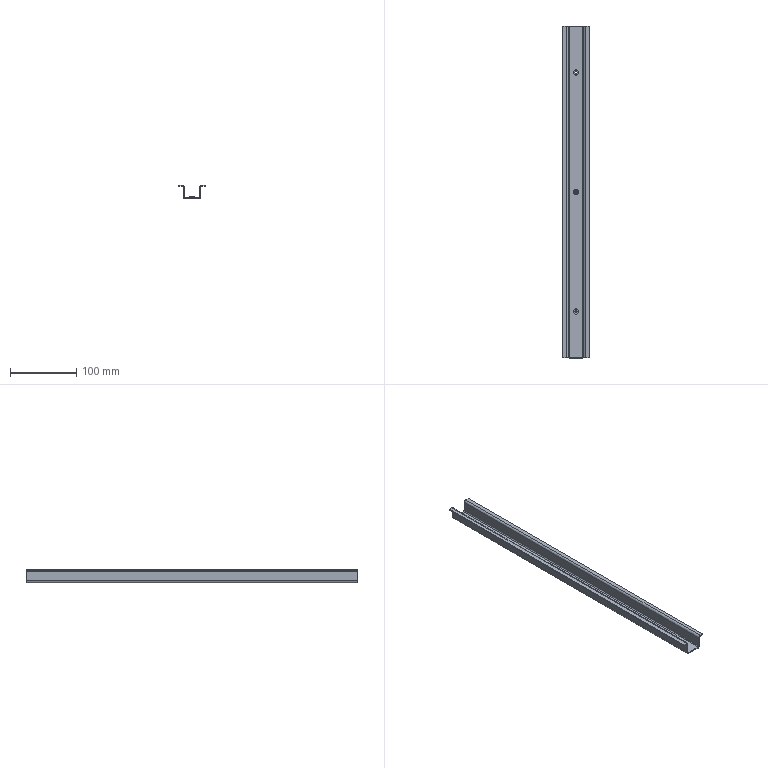Part | SolidWorks | features 3DProfileFeature 1, FlatPattern 1, HoleWzd 1, ICE 1, SMBaseFlange 1, SheetMetal 1 | 1 solid | 53 faces | box 40 x 500 x 21 mm | volume 56565 mm3 | plane 33 | cylinder 20 | commonest cylinder face diameters 3.3 x6 8 x6 3 x4 6 x4
STEP:
#1=CARTESIAN_POINT('',(-1.65,180.,-19.5));
#2=VERTEX_POINT('',#1);
#3=CARTESIAN_POINT('',(1.65,180.,-19.5));
#4=VERTEX_POINT('',#3);
#5=CARTESIAN_POINT('',(0.,180.,-19.5));
#6=DIRECTION('',(0.,0.,1.));
#7=DIRECTION('',(1.,0.,0.));
#8=AXIS2_PLACEMENT_3D('',#5,#6,#7);
#9=CIRCLE('',#8,1.65);
#10=EDGE_CURVE('',#2,#4,#9,.T.);
#11=ORIENTED_EDGE('',*,*,#10,.F.);
#12=CARTESIAN_POINT('',(-1.65,180.,-16.));
#13=VERTEX_POINT('',#12);
#14=CARTESIAN_POINT('',(-1.65,180.,-16.));
#15=DIRECTION('',(0.,0.,1.));
#16=VECTOR('',#15,1000.);
#17=LINE('',#14,#16);
#18=EDGE_CURVE('',#2,#13,#17,.T.);
#19=ORIENTED_EDGE('',*,*,#18,.T.);
#20=CARTESIAN_POINT('',(1.65,180.,-16.));
#21=VERTEX_POINT('',#20);
#22=CARTESIAN_POINT('',(0.,180.,-16.));
#23=DIRECTION('',(0.,0.,1.));
#24=DIRECTION('',(1.,0.,0.));
#25=AXIS2_PLACEMENT_3D('',#22,#23,#24);
#26=CIRCLE('',#25,1.65);
#27=EDGE_CURVE('',#13,#21,#26,.T.);
#28=ORIENTED_EDGE('',*,*,#27,.T.);
#29=CARTESIAN_POINT('',(1.65,180.,-16.));
#30=DIRECTION('',(0.,0.,1.));
#31=VECTOR('',#30,1000.);
#32=LINE('',#29,#31);
#33=EDGE_CURVE('',#4,#21,#32,.T.);
#34=ORIENTED_EDGE('',*,*,#33,.F.);
#35=EDGE_LOOP('',(#11,#19,#28,#34));
#36=FACE_OUTER_BOUND('',#35,.T.);
#37=CARTESIAN_POINT('',(0.,180.,-16.));
#38=DIRECTION('',(0.,0.,1.));
#39=DIRECTION('',(1.,0.,0.));
#40=AXIS2_PLACEMENT_3D('',#37,#38,#39);
#41=CYLINDRICAL_SURFACE('',#40,1.65);
#42=ADVANCED_FACE('',(#36),#41,.F.);
#43=CARTESIAN_POINT('',(-1.65,0.,-19.5));
#44=VERTEX_POINT('',#43);
#45=CARTESIAN_POINT('',(1.65,0.,-19.5));
#46=VERTEX_POINT('',#45);
#47=CARTESIAN_POINT('',(0.,0.,-19.5));
#48=DIRECTION('',(0.,0.,1.));
#49=DIRECTION('',(1.,0.,0.));
#50=AXIS2_PLACEMENT_3D('',#47,#48,#49);
#51=CIRCLE('',#50,1.65);
#52=EDGE_CURVE('',#44,#46,#51,.T.);
#53=ORIENTED_EDGE('',*,*,#52,.F.);
#54=CARTESIAN_POINT('',(-1.65,0.,-16.));
#55=VERTEX_POINT('',#54);
#56=CARTESIAN_POINT('',(-1.65,0.,-16.));
#57=DIRECTION('',(0.,0.,1.));
#58=VECTOR('',#57,1000.);
#59=LINE('',#56,#58);
#60=EDGE_CURVE('',#44,#55,#59,.T.);
#61=ORIENTED_EDGE('',*,*,#60,.T.);
#62=CARTESIAN_POINT('',(1.65,0.,-16.));
#63=VERTEX_POINT('',#62);
#64=CARTESIAN_POINT('',(0.,0.,-16.));
#65=DIRECTION('',(0.,0.,1.));
#66=DIRECTION('',(1.,0.,0.));
#67=AXIS2_PLACEMENT_3D('',#64,#65,#66);
#68=CIRCLE('',#67,1.65);
#69=EDGE_CURVE('',#55,#63,#68,.T.);
#70=ORIENTED_EDGE('',*,*,#69,.T.);
#71=CARTESIAN_POINT('',(1.65,0.,-16.));
#72=DIRECTION('',(0.,0.,1.));
#73=VECTOR('',#72,1000.);
#74=LINE('',#71,#73);
#75=EDGE_CURVE('',#46,#63,#74,.T.);
#76=ORIENTED_EDGE('',*,*,#75,.F.);
#77=EDGE_LOOP('',(#53,#61,#70,#76));
#78=FACE_OUTER_BOUND('',#77,.T.);
#79=CARTESIAN_POINT('',(0.,0.,-16.));
#80=DIRECTION('',(0.,0.,1.));
#81=DIRECTION('',(1.,0.,0.));
#82=AXIS2_PLACEMENT_3D('',#79,#80,#81);
#83=CYLINDRICAL_SURFACE('',#82,1.65);
#84=ADVANCED_FACE('',(#78),#83,.F.);
#85=CARTESIAN_POINT('',(-1.65,-180.,-19.5));
#86=VERTEX_POINT('',#85);
#87=CARTESIAN_POINT('',(1.65,-180.,-19.5));
#88=VERTEX_POINT('',#87);
#89=CARTESIAN_POINT('',(0.,-180.,-19.5));
#90=DIRECTION('',(0.,0.,1.));
#91=DIRECTION('',(1.,0.,0.));
#92=AXIS2_PLACEMENT_3D('',#89,#90,#91);
#93=CIRCLE('',#92,1.65);
#94=EDGE_CURVE('',#86,#88,#93,.T.);
#95=ORIENTED_EDGE('',*,*,#94,.F.);
#96=CARTESIAN_POINT('',(-1.65,-180.,-16.));
#97=VERTEX_POINT('',#96);
#98=CARTESIAN_POINT('',(-1.65,-180.,-16.));
#99=DIRECTION('',(0.,0.,1.));
#100=VECTOR('',#99,1000.);
#101=LINE('',#98,#100);
#102=EDGE_CURVE('',#86,#97,#101,.T.);
#103=ORIENTED_EDGE('',*,*,#102,.T.);
#104=CARTESIAN_POINT('',(1.65,-180.,-16.));
#105=VERTEX_POINT('',#104);
#106=CARTESIAN_POINT('',(0.,-180.,-16.));
#107=DIRECTION('',(0.,0.,1.));
#108=DIRECTION('',(1.,0.,0.));
#109=AXIS2_PLACEMENT_3D('',#106,#107,#108);
#110=CIRCLE('',#109,1.65);
#111=EDGE_CURVE('',#97,#105,#110,.T.);
#112=ORIENTED_EDGE('',*,*,#111,.T.);
#113=CARTESIAN_POINT('',(1.65,-180.,-16.));
#114=DIRECTION('',(0.,0.,1.));
#115=VECTOR('',#114,1000.);
#116=LINE('',#113,#115);
#117=EDGE_CURVE('',#88,#105,#116,.T.);
#118=ORIENTED_EDGE('',*,*,#117,.F.);
#119=EDGE_LOOP('',(#95,#103,#112,#118));
#120=FACE_OUTER_BOUND('',#119,.T.);
#121=CARTESIAN_POINT('',(0.,-180.,-16.));
#122=DIRECTION('',(0.,0.,1.));
#123=DIRECTION('',(1.,0.,0.));
#124=AXIS2_PLACEMENT_3D('',#121,#122,#123);
#125=CYLINDRICAL_SURFACE('',#124,1.65);
#126=ADVANCED_FACE('',(#120),#125,.F.);
#127=CARTESIAN_POINT('',(-4.,-180.,-16.));
#128=VERTEX_POINT('',#127);
#129=CARTESIAN_POINT('',(4.,-180.,-16.));
#130=VERTEX_POINT('',#129);
#131=CARTESIAN_POINT('',(0.,-180.,-16.));
#132=DIRECTION('',(0.,0.,-1.));
#133=DIRECTION('',(1.,0.,0.));
#134=AXIS2_PLACEMENT_3D('',#131,#132,#133);
#135=CIRCLE('',#134,4.);
#136=EDGE_CURVE('',#128,#130,#135,.T.);
#137=ORIENTED_EDGE('',*,*,#136,.T.);
#138=CARTESIAN_POINT('',(4.,-180.,-18.));
#139=VERTEX_POINT('',#138);
#140=CARTESIAN_POINT('',(4.,-180.,-16.));
#141=DIRECTION('',(0.,0.,-1.));
#142=VECTOR('',#141,1000.);
#143=LINE('',#140,#142);
#144=EDGE_CURVE('',#130,#139,#143,.T.);
#145=ORIENTED_EDGE('',*,*,#144,.T.);
#146=CARTESIAN_POINT('',(-4.,-180.,-18.));
#147=VERTEX_POINT('',#146);
#148=CARTESIAN_POINT('',(0.,-180.,-18.));
#149=DIRECTION('',(0.,0.,-1.));
#150=DIRECTION('',(1.,0.,0.));
#151=AXIS2_PLACEMENT_3D('',#148,#149,#150);
#152=CIRCLE('',#151,4.);
#153=EDGE_CURVE('',#147,#139,#152,.T.);
#154=ORIENTED_EDGE('',*,*,#153,.F.);
#155=CARTESIAN_POINT('',(-4.,-180.,-16.));
#156=DIRECTION('',(0.,0.,-1.));
#157=VECTOR('',#156,1000.);
#158=LINE('',#155,#157);
#159=EDGE_CURVE('',#128,#147,#158,.T.);
#160=ORIENTED_EDGE('',*,*,#159,.F.);
#161=EDGE_LOOP('',(#137,#145,#154,#160));
#162=FACE_OUTER_BOUND('',#161,.T.);
#163=CARTESIAN_POINT('',(0.,-180.,-16.));
#164=DIRECTION('',(0.,0.,-1.));
#165=DIRECTION('',(-1.,0.,0.));
#166=AXIS2_PLACEMENT_3D('',#163,#164,#165);
#167=CYLINDRICAL_SURFACE('',#166,4.);
#168=ADVANCED_FACE('',(#162),#167,.T.);
#169=CARTESIAN_POINT('',(4.,0.,-16.));
#170=VERTEX_POINT('',#169);
#171=CARTESIAN_POINT('',(-4.,0.,-16.));
#172=VERTEX_POINT('',#171);
#173=CARTESIAN_POINT('',(0.,0.,-16.));
#174=DIRECTION('',(0.,0.,1.));
#175=DIRECTION('',(1.,0.,0.));
#176=AXIS2_PLACEMENT_3D('',#173,#174,#175);
#177=CIRCLE('',#176,4.);
#178=EDGE_CURVE('',#170,#172,#177,.T.);
#179=ORIENTED_EDGE('',*,*,#178,.F.);
#180=CARTESIAN_POINT('',(4.,0.,-18.));
#181=VERTEX_POINT('',#180);
#182=CARTESIAN_POINT('',(4.,0.,-16.));
#183=DIRECTION('',(0.,0.,-1.));
#184=VECTOR('',#183,1000.);
#185=LINE('',#182,#184);
#186=EDGE_CURVE('',#170,#181,#185,.T.);
#187=ORIENTED_EDGE('',*,*,#186,.T.);
#188=CARTESIAN_POINT('',(-4.,0.,-18.));
#189=VERTEX_POINT('',#188);
#190=CARTESIAN_POINT('',(0.,0.,-18.));
#191=DIRECTION('',(0.,0.,1.));
#192=DIRECTION('',(-1.,0.,0.));
#193=AXIS2_PLACEMENT_3D('',#190,#191,#192);
#194=CIRCLE('',#193,4.);
#195=EDGE_CURVE('',#181,#189,#194,.T.);
#196=ORIENTED_EDGE('',*,*,#195,.T.);
#197=CARTESIAN_POINT('',(-4.,0.,-16.));
#198=DIRECTION('',(0.,0.,-1.));
#199=VECTOR('',#198,1000.);
#200=LINE('',#197,#199);
#201=EDGE_CURVE('',#172,#189,#200,.T.);
#202=ORIENTED_EDGE('',*,*,#201,.F.);
#203=EDGE_LOOP('',(#179,#187,#196,#202));
#204=FACE_OUTER_BOUND('',#203,.T.);
#205=CARTESIAN_POINT('',(0.,0.,-16.));
#206=DIRECTION('',(0.,0.,-1.));
#207=DIRECTION('',(-1.,0.,0.));
#208=AXIS2_PLACEMENT_3D('',#205,#206,#207);
#209=CYLINDRICAL_SURFACE('',#208,4.);
#210=ADVANCED_FACE('',(#204),#209,.T.);
#211=CARTESIAN_POINT('',(4.,180.,-16.));
#212=VERTEX_POINT('',#211);
#213=CARTESIAN_POINT('',(-4.,180.,-16.));
#214=VERTEX_POINT('',#213);
#215=CARTESIAN_POINT('',(0.,180.,-16.));
#216=DIRECTION('',(0.,0.,1.));
#217=DIRECTION('',(1.,0.,0.));
#218=AXIS2_PLACEMENT_3D('',#215,#216,#217);
#219=CIRCLE('',#218,4.);
#220=EDGE_CURVE('',#212,#214,#219,.T.);
#221=ORIENTED_EDGE('',*,*,#220,.F.);
#222=CARTESIAN_POINT('',(4.,180.,-18.));
#223=VERTEX_POINT('',#222);
#224=CARTESIAN_POINT('',(4.,180.,-16.));
#225=DIRECTION('',(0.,0.,-1.));
#226=VECTOR('',#225,1000.);
#227=LINE('',#224,#226);
#228=EDGE_CURVE('',#212,#223,#227,.T.);
#229=ORIENTED_EDGE('',*,*,#228,.T.);
#230=CARTESIAN_POINT('',(-4.,180.,-18.));
#231=VERTEX_POINT('',#230);
#232=CARTESIAN_POINT('',(0.,180.,-18.));
#233=DIRECTION('',(0.,0.,1.));
#234=DIRECTION('',(-1.,0.,0.));
#235=AXIS2_PLACEMENT_3D('',#232,#233,#234);
#236=CIRCLE('',#235,4.);
#237=EDGE_CURVE('',#223,#231,#236,.T.);
#238=ORIENTED_EDGE('',*,*,#237,.T.);
#239=CARTESIAN_POINT('',(-4.,180.,-16.));
#240=DIRECTION('',(0.,0.,-1.));
#241=VECTOR('',#240,1000.);
#242=LINE('',#239,#241);
#243=EDGE_CURVE('',#214,#231,#242,.T.);
#244=ORIENTED_EDGE('',*,*,#243,.F.);
#245=EDGE_LOOP('',(#221,#229,#238,#244));
#246=FACE_OUTER_BOUND('',#245,.T.);
#247=CARTESIAN_POINT('',(0.,180.,-16.));
#248=DIRECTION('',(0.,0.,-1.));
#249=DIRECTION('',(-1.,0.,0.));
#250=AXIS2_PLACEMENT_3D('',#247,#248,#249);
#251=CYLINDRICAL_SURFACE('',#250,4.);
#252=ADVANCED_FACE('',(#246),#251,.T.);
#253=CARTESIAN_POINT('',(-13.,250.,-1.5));
#254=VERTEX_POINT('',#253);
#255=CARTESIAN_POINT('',(-11.5,250.,-1.5));
#256=VERTEX_POINT('',#255);
#257=CARTESIAN_POINT('',(-13.,250.,-1.5));
#258=DIRECTION('',(1.,0.,0.));
#259=VECTOR('',#258,1000.);
#260=LINE('',#257,#259);
#261=EDGE_CURVE('',#254,#256,#260,.T.);
#262=ORIENTED_EDGE('',*,*,#261,.F.);
#263=CARTESIAN_POINT('',(-14.5,250.,0.));
#264=VERTEX_POINT('',#263);
#265=CARTESIAN_POINT('',(-14.5,250.,-1.5));
#266=DIRECTION('',(0.,1.,0.));
#267=DIRECTION('',(0.,0.,-1.));
#268=AXIS2_PLACEMENT_3D('',#265,#266,#267);
#269=CIRCLE('',#268,1.5);
#270=EDGE_CURVE('',#264,#254,#269,.T.);
#271=ORIENTED_EDGE('',*,*,#270,.F.);
#272=CARTESIAN_POINT('',(-14.5,250.,1.5));
#273=VERTEX_POINT('',#272);
#274=CARTESIAN_POINT('',(-14.5,250.,1.5));
#275=DIRECTION('',(0.,0.,-1.));
#276=VECTOR('',#275,1000.);
#277=LINE('',#274,#276);
#278=EDGE_CURVE('',#273,#264,#277,.T.);
#279=ORIENTED_EDGE('',*,*,#278,.F.);
#280=CARTESIAN_POINT('',(-14.5,250.,-1.5));
#281=DIRECTION('',(0.,1.,0.));
#282=DIRECTION('',(1.,0.,0.));
#283=AXIS2_PLACEMENT_3D('',#280,#281,#282);
#284=CIRCLE('',#283,3.);
#285=EDGE_CURVE('',#273,#256,#284,.T.);
#286=ORIENTED_EDGE('',*,*,#285,.T.);
#287=EDGE_LOOP('',(#262,#271,#279,#286));
#288=FACE_OUTER_BOUND('',#287,.T.);
#289=CARTESIAN_POINT('',(-13.,250.,-1.5));
#290=DIRECTION('',(0.,1.,0.));
#291=DIRECTION('',(0.,0.,1.));
#292=AXIS2_PLACEMENT_3D('',#289,#290,#291);
#293=PLANE('',#292);
#294=ADVANCED_FACE('',(#288),#293,.T.);
#295=CARTESIAN_POINT('',(-13.,250.,-16.5));
#296=VERTEX_POINT('',#295);
#297=CARTESIAN_POINT('',(-13.,250.,0.));
#298=DIRECTION('',(0.,0.,-1.));
#299=VECTOR('',#298,1000.);
#300=LINE('',#297,#299);
#301=EDGE_CURVE('',#254,#296,#300,.T.);
#302=ORIENTED_EDGE('',*,*,#301,.F.);
#303=ORIENTED_EDGE('',*,*,#261,.T.);
#304=CARTESIAN_POINT('',(-11.5,250.,-16.5));
#305=VERTEX_POINT('',#304);
#306=CARTESIAN_POINT('',(-11.5,250.,0.));
#307=DIRECTION('',(0.,0.,-1.));
#308=VECTOR('',#307,1000.);
#309=LINE('',#306,#308);
#310=EDGE_CURVE('',#256,#305,#309,.T.);
#311=ORIENTED_EDGE('',*,*,#310,.T.);
#312=CARTESIAN_POINT('',(-11.5,250.,-16.5));
#313=DIRECTION('',(-1.,0.,0.));
#314=VECTOR('',#313,1000.);
#315=LINE('',#312,#314);
#316=EDGE_CURVE('',#305,#296,#315,.T.);
#317=ORIENTED_EDGE('',*,*,#316,.T.);
#318=EDGE_LOOP('',(#302,#303,#311,#317));
#319=FACE_OUTER_BOUND('',#318,.T.);
#320=CARTESIAN_POINT('',(-14.5,250.,1.5));
#321=DIRECTION('',(0.,1.,0.));
#322=DIRECTION('',(0.,0.,1.));
#323=AXIS2_PLACEMENT_3D('',#320,#321,#322);
#324=PLANE('',#323);
#325=ADVANCED_FACE('',(#319),#324,.T.);
#326=CARTESIAN_POINT('',(-14.5,-250.,0.));
#327=VERTEX_POINT('',#326);
#328=CARTESIAN_POINT('',(-14.5,-250.,1.5));
#329=VERTEX_POINT('',#328);
#330=CARTESIAN_POINT('',(-14.5,-250.,0.));
#331=DIRECTION('',(0.,0.,1.));
#332=VECTOR('',#331,1000.);
#333=LINE('',#330,#332);
#334=EDGE_CURVE('',#327,#329,#333,.T.);
#335=ORIENTED_EDGE('',*,*,#334,.F.);
#336=CARTESIAN_POINT('',(-13.,-250.,-1.5));
#337=VERTEX_POINT('',#336);
#338=CARTESIAN_POINT('',(-14.5,-250.,-1.5));
#339=DIRECTION('',(0.,1.,0.));
#340=DIRECTION('',(0.,0.,-1.));
#341=AXIS2_PLACEMENT_3D('',#338,#339,#340);
#342=CIRCLE('',#341,1.5);
#343=EDGE_CURVE('',#327,#337,#342,.T.);
#344=ORIENTED_EDGE('',*,*,#343,.T.);
#345=CARTESIAN_POINT('',(-11.5,-250.,-1.5));
#346=VERTEX_POINT('',#345);
#347=CARTESIAN_POINT('',(-11.5,-250.,-1.5));
#348=DIRECTION('',(-1.,0.,0.));
#349=VECTOR('',#348,1000.);
#350=LINE('',#347,#349);
#351=EDGE_CURVE('',#346,#337,#350,.T.);
#352=ORIENTED_EDGE('',*,*,#351,.F.);
#353=CARTESIAN_POINT('',(-14.5,-250.,-1.5));
#354=DIRECTION('',(0.,1.,0.));
#355=DIRECTION('',(1.,0.,0.));
#356=AXIS2_PLACEMENT_3D('',#353,#354,#355);
#357=CIRCLE('',#356,3.);
#358=EDGE_CURVE('',#329,#346,#357,.T.);
#359=ORIENTED_EDGE('',*,*,#358,.F.);
#360=EDGE_LOOP('',(#335,#344,#352,#359));
#361=FACE_OUTER_BOUND('',#360,.T.);
#362=CARTESIAN_POINT('',(-14.5,-250.,0.));
#363=DIRECTION('',(0.,-1.,0.));
#364=DIRECTION('',(0.,0.,-1.));
#365=AXIS2_PLACEMENT_3D('',#362,#363,#364);
#366=PLANE('',#365);
#367=ADVANCED_FACE('',(#361),#366,.T.);
#368=CARTESIAN_POINT('',(-20.,-250.,0.));
#369=VERTEX_POINT('',#368);
#370=CARTESIAN_POINT('',(-20.,-250.,0.));
#371=DIRECTION('',(1.,0.,0.));
#372=VECTOR('',#371,1000.);
#373=LINE('',#370,#372);
#374=EDGE_CURVE('',#369,#327,#373,.T.);
#375=ORIENTED_EDGE('',*,*,#374,.T.);
#376=ORIENTED_EDGE('',*,*,#334,.T.);
#377=CARTESIAN_POINT('',(-20.,-250.,1.5));
#378=VERTEX_POINT('',#377);
#379=CARTESIAN_POINT('',(-20.,-250.,1.5));
#380=DIRECTION('',(1.,0.,0.));
#381=VECTOR('',#380,1000.);
#382=LINE('',#379,#381);
#383=EDGE_CURVE('',#378,#329,#382,.T.);
#384=ORIENTED_EDGE('',*,*,#383,.F.);
#385=CARTESIAN_POINT('',(-20.,-250.,1.5));
#386=DIRECTION('',(0.,0.,-1.));
#387=VECTOR('',#386,1000.);
#388=LINE('',#385,#387);
#389=EDGE_CURVE('',#378,#369,#388,.T.);
#390=ORIENTED_EDGE('',*,*,#389,.T.);
#391=EDGE_LOOP('',(#375,#376,#384,#390));
#392=FACE_OUTER_BOUND('',#391,.T.);
#393=CARTESIAN_POINT('',(-11.5,-250.,-1.5));
#394=DIRECTION('',(0.,-1.,0.));
#395=DIRECTION('',(0.,0.,-1.));
#396=AXIS2_PLACEMENT_3D('',#393,#394,#395);
#397=PLANE('',#396);
#398=ADVANCED_FACE('',(#392),#397,.T.);
#399=CARTESIAN_POINT('',(-10.,250.,-19.5));
#400=VERTEX_POINT('',#399);
#401=CARTESIAN_POINT('',(-10.,250.,-18.));
#402=VERTEX_POINT('',#401);
#403=CARTESIAN_POINT('',(-10.,250.,-19.5));
#404=DIRECTION('',(0.,0.,1.));
#405=VECTOR('',#404,1000.);
#406=LINE('',#403,#405);
#407=EDGE_CURVE('',#400,#402,#406,.T.);
#408=ORIENTED_EDGE('',*,*,#407,.F.);
#409=CARTESIAN_POINT('',(-10.,250.,-16.5));
#410=DIRECTION('',(0.,-1.,0.));
#411=DIRECTION('',(0.,0.,1.));
#412=AXIS2_PLACEMENT_3D('',#409,#410,#411);
#413=CIRCLE('',#412,3.);
#414=EDGE_CURVE('',#296,#400,#413,.T.);
#415=ORIENTED_EDGE('',*,*,#414,.F.);
#416=ORIENTED_EDGE('',*,*,#316,.F.);
#417=CARTESIAN_POINT('',(-10.,250.,-16.5));
#418=DIRECTION('',(0.,-1.,0.));
#419=DIRECTION('',(1.,0.,0.));
#420=AXIS2_PLACEMENT_3D('',#417,#418,#419);
#421=CIRCLE('',#420,1.5);
#422=EDGE_CURVE('',#305,#402,#421,.T.);
#423=ORIENTED_EDGE('',*,*,#422,.T.);
#424=EDGE_LOOP('',(#408,#415,#416,#423));
#425=FACE_OUTER_BOUND('',#424,.T.);
#426=CARTESIAN_POINT('',(-10.,250.,-19.5));
#427=DIRECTION('',(0.,1.,0.));
#428=DIRECTION('',(0.,0.,1.));
#429=AXIS2_PLACEMENT_3D('',#426,#427,#428);
#430=PLANE('',#429);
#431=ADVANCED_FACE('',(#425),#430,.T.);
#432=CARTESIAN_POINT('',(10.,250.,-19.5));
#433=VERTEX_POINT('',#432);
#434=CARTESIAN_POINT('',(-13.,250.,-19.5));
#435=DIRECTION('',(1.,0.,0.));
#436=VECTOR('',#435,1000.);
#437=LINE('',#434,#436);
#438=EDGE_CURVE('',#400,#433,#437,.T.);
#439=ORIENTED_EDGE('',*,*,#438,.F.);
#440=ORIENTED_EDGE('',*,*,#407,.T.);
#441=CARTESIAN_POINT('',(10.,250.,-18.));
#442=VERTEX_POINT('',#441);
#443=CARTESIAN_POINT('',(-13.,250.,-18.));
#444=DIRECTION('',(1.,0.,0.));
#445=VECTOR('',#444,1000.);
#446=LINE('',#443,#445);
#447=EDGE_CURVE('',#402,#442,#446,.T.);
#448=ORIENTED_EDGE('',*,*,#447,.T.);
#449=CARTESIAN_POINT('',(10.,250.,-18.));
#450=DIRECTION('',(0.,0.,-1.));
#451=VECTOR('',#450,1000.);
#452=LINE('',#449,#451);
#453=EDGE_CURVE('',#442,#433,#452,.T.);
#454=ORIENTED_EDGE('',*,*,#453,.T.);
#455=EDGE_LOOP('',(#439,#440,#448,#454));
#456=FACE_OUTER_BOUND('',#455,.T.);
#457=CARTESIAN_POINT('',(-11.5,250.,-16.5));
#458=DIRECTION('',(0.,1.,0.));
#459=DIRECTION('',(0.,0.,1.));
#460=AXIS2_PLACEMENT_3D('',#457,#458,#459);
#461=PLANE('',#460);
#462=ADVANCED_FACE('',(#456),#461,.T.);
#463=CARTESIAN_POINT('',(-13.,-250.,-16.5));
#464=VERTEX_POINT('',#463);
#465=CARTESIAN_POINT('',(-11.5,-250.,-16.5));
#466=VERTEX_POINT('',#465);
#467=CARTESIAN_POINT('',(-13.,-250.,-16.5));
#468=DIRECTION('',(1.,0.,0.));
#469=VECTOR('',#468,1000.);
#470=LINE('',#467,#469);
#471=EDGE_CURVE('',#464,#466,#470,.T.);
#472=ORIENTED_EDGE('',*,*,#471,.F.);
#473=CARTESIAN_POINT('',(-10.,-250.,-19.5));
#474=VERTEX_POINT('',#473);
#475=CARTESIAN_POINT('',(-10.,-250.,-16.5));
#476=DIRECTION('',(0.,-1.,0.));
#477=DIRECTION('',(0.,0.,1.));
#478=AXIS2_PLACEMENT_3D('',#475,#476,#477);
#479=CIRCLE('',#478,3.);
#480=EDGE_CURVE('',#464,#474,#479,.T.);
#481=ORIENTED_EDGE('',*,*,#480,.T.);
#482=CARTESIAN_POINT('',(-10.,-250.,-18.));
#483=VERTEX_POINT('',#482);
#484=CARTESIAN_POINT('',(-10.,-250.,-18.));
#485=DIRECTION('',(0.,0.,-1.));
#486=VECTOR('',#485,1000.);
#487=LINE('',#484,#486);
#488=EDGE_CURVE('',#483,#474,#487,.T.);
#489=ORIENTED_EDGE('',*,*,#488,.F.);
#490=CARTESIAN_POINT('',(-10.,-250.,-16.5));
#491=DIRECTION('',(0.,-1.,0.));
#492=DIRECTION('',(1.,0.,0.));
#493=AXIS2_PLACEMENT_3D('',#490,#491,#492);
#494=CIRCLE('',#493,1.5);
#495=EDGE_CURVE('',#466,#483,#494,.T.);
#496=ORIENTED_EDGE('',*,*,#495,.F.);
#497=EDGE_LOOP('',(#472,#481,#489,#496));
#498=FACE_OUTER_BOUND('',#497,.T.);
#499=CARTESIAN_POINT('',(-13.,-250.,-16.5));
#500=DIRECTION('',(0.,-1.,0.));
#501=DIRECTION('',(0.,0.,-1.));
#502=AXIS2_PLACEMENT_3D('',#499,#500,#501);
#503=PLANE('',#502);
#504=ADVANCED_FACE('',(#498),#503,.T.);
#505=CARTESIAN_POINT('',(-13.,-250.,0.));
#506=DIRECTION('',(0.,0.,-1.));
#507=VECTOR('',#506,1000.);
#508=LINE('',#505,#507);
#509=EDGE_CURVE('',#337,#464,#508,.T.);
#510=ORIENTED_EDGE('',*,*,#509,.T.);
#511=ORIENTED_EDGE('',*,*,#471,.T.);
#512=CARTESIAN_POINT('',(-11.5,-250.,0.));
#513=DIRECTION('',(0.,0.,-1.));
#514=VECTOR('',#513,1000.);
#515=LINE('',#512,#514);
#516=EDGE_CURVE('',#346,#466,#515,.T.);
#517=ORIENTED_EDGE('',*,*,#516,.F.);
#518=ORIENTED_EDGE('',*,*,#351,.T.);
#519=EDGE_LOOP('',(#510,#511,#517,#518));
#520=FACE_OUTER_BOUND('',#519,.T.);
#521=CARTESIAN_POINT('',(-10.,-250.,-18.));
#522=DIRECTION('',(0.,-1.,0.));
#523=DIRECTION('',(0.,0.,-1.));
#524=AXIS2_PLACEMENT_3D('',#521,#522,#523);
#525=PLANE('',#524);
#526=ADVANCED_FACE('',(#520),#525,.T.);
#527=CARTESIAN_POINT('',(13.,250.,-16.5));
#528=VERTEX_POINT('',#527);
#529=CARTESIAN_POINT('',(11.5,250.,-16.5));
#530=VERTEX_POINT('',#529);
#531=CARTESIAN_POINT('',(13.,250.,-16.5));
#532=DIRECTION('',(-1.,0.,0.));
#533=VECTOR('',#532,1000.);
#534=LINE('',#531,#533);
#535=EDGE_CURVE('',#528,#530,#534,.T.);
#536=ORIENTED_EDGE('',*,*,#535,.F.);
#537=CARTESIAN_POINT('',(10.,250.,-16.5));
#538=DIRECTION('',(0.,-1.,0.));
#539=DIRECTION('',(0.,0.,1.));
#540=AXIS2_PLACEMENT_3D('',#537,#538,#539);
#541=CIRCLE('',#540,3.);
#542=EDGE_CURVE('',#433,#528,#541,.T.);
#543=ORIENTED_EDGE('',*,*,#542,.F.);
#544=ORIENTED_EDGE('',*,*,#453,.F.);
#545=CARTESIAN_POINT('',(10.,250.,-16.5));
#546=DIRECTION('',(0.,-1.,0.));
#547=DIRECTION('',(1.,0.,0.));
#548=AXIS2_PLACEMENT_3D('',#545,#546,#547);
#549=CIRCLE('',#548,1.5);
#550=EDGE_CURVE('',#442,#530,#549,.T.);
#551=ORIENTED_EDGE('',*,*,#550,.T.);
#552=EDGE_LOOP('',(#536,#543,#544,#551));
#553=FACE_OUTER_BOUND('',#552,.T.);
#554=CARTESIAN_POINT('',(13.,250.,-16.5));
#555=DIRECTION('',(0.,1.,0.));
#556=DIRECTION('',(0.,0.,1.));
#557=AXIS2_PLACEMENT_3D('',#554,#555,#556);
#558=PLANE('',#557);
#559=ADVANCED_FACE('',(#553),#558,.T.);
#560=CARTESIAN_POINT('',(13.,250.,-1.5));
#561=VERTEX_POINT('',#560);
#562=CARTESIAN_POINT('',(13.,250.,-19.5));
#563=DIRECTION('',(0.,0.,1.));
#564=VECTOR('',#563,1000.);
#565=LINE('',#562,#564);
#566=EDGE_CURVE('',#528,#561,#565,.T.);
#567=ORIENTED_EDGE('',*,*,#566,.F.);
#568=ORIENTED_EDGE('',*,*,#535,.T.);
#569=CARTESIAN_POINT('',(11.5,250.,-1.5));
#570=VERTEX_POINT('',#569);
#571=CARTESIAN_POINT('',(11.5,250.,-19.5));
#572=DIRECTION('',(0.,0.,1.));
#573=VECTOR('',#572,1000.);
#574=LINE('',#571,#573);
#575=EDGE_CURVE('',#530,#570,#574,.T.);
#576=ORIENTED_EDGE('',*,*,#575,.T.);
#577=CARTESIAN_POINT('',(11.5,250.,-1.5));
#578=DIRECTION('',(1.,0.,0.));
#579=VECTOR('',#578,1000.);
#580=LINE('',#577,#579);
#581=EDGE_CURVE('',#570,#561,#580,.T.);
#582=ORIENTED_EDGE('',*,*,#581,.T.);
#583=EDGE_LOOP('',(#567,#568,#576,#582));
#584=FACE_OUTER_BOUND('',#583,.T.);
#585=CARTESIAN_POINT('',(10.,250.,-18.));
#586=DIRECTION('',(0.,1.,0.));
#587=DIRECTION('',(0.,0.,1.));
#588=AXIS2_PLACEMENT_3D('',#585,#586,#587);
#589=PLANE('',#588);
#590=ADVANCED_FACE('',(#584),#589,.T.);
#591=CARTESIAN_POINT('',(10.,-250.,-19.5));
#592=VERTEX_POINT('',#591);
#593=CARTESIAN_POINT('',(10.,-250.,-18.));
#594=VERTEX_POINT('',#593);
#595=CARTESIAN_POINT('',(10.,-250.,-19.5));
#596=DIRECTION('',(0.,0.,1.));
#597=VECTOR('',#596,1000.);
#598=LINE('',#595,#597);
#599=EDGE_CURVE('',#592,#594,#598,.T.);
#600=ORIENTED_EDGE('',*,*,#599,.F.);
#601=CARTESIAN_POINT('',(13.,-250.,-16.5));
#602=VERTEX_POINT('',#601);
#603=CARTESIAN_POINT('',(10.,-250.,-16.5));
#604=DIRECTION('',(0.,-1.,0.));
#605=DIRECTION('',(0.,0.,1.));
#606=AXIS2_PLACEMENT_3D('',#603,#604,#605);
#607=CIRCLE('',#606,3.);
#608=EDGE_CURVE('',#592,#602,#607,.T.);
#609=ORIENTED_EDGE('',*,*,#608,.T.);
#610=CARTESIAN_POINT('',(11.5,-250.,-16.5));
#611=VERTEX_POINT('',#610);
#612=CARTESIAN_POINT('',(11.5,-250.,-16.5));
#613=DIRECTION('',(1.,0.,0.));
#614=VECTOR('',#613,1000.);
#615=LINE('',#612,#614);
#616=EDGE_CURVE('',#611,#602,#615,.T.);
#617=ORIENTED_EDGE('',*,*,#616,.F.);
#618=CARTESIAN_POINT('',(10.,-250.,-16.5));
#619=DIRECTION('',(0.,-1.,0.));
#620=DIRECTION('',(1.,0.,0.));
#621=AXIS2_PLACEMENT_3D('',#618,#619,#620);
#622=CIRCLE('',#621,1.5);
#623=EDGE_CURVE('',#594,#611,#622,.T.);
#624=ORIENTED_EDGE('',*,*,#623,.F.);
#625=EDGE_LOOP('',(#600,#609,#617,#624));
#626=FACE_OUTER_BOUND('',#625,.T.);
#627=CARTESIAN_POINT('',(10.,-250.,-19.5));
#628=DIRECTION('',(0.,-1.,0.));
#629=DIRECTION('',(0.,0.,-1.));
#630=AXIS2_PLACEMENT_3D('',#627,#628,#629);
#631=PLANE('',#630);
#632=ADVANCED_FACE('',(#626),#631,.T.);
#633=CARTESIAN_POINT('',(-13.,-250.,-19.5));
#634=DIRECTION('',(1.,0.,0.));
#635=VECTOR('',#634,1000.);
#636=LINE('',#633,#635);
#637=EDGE_CURVE('',#474,#592,#636,.T.);
#638=ORIENTED_EDGE('',*,*,#637,.T.);
#639=ORIENTED_EDGE('',*,*,#599,.T.);
#640=CARTESIAN_POINT('',(-13.,-250.,-18.));
#641=DIRECTION('',(1.,0.,0.));
#642=VECTOR('',#641,1000.);
#643=LINE('',#640,#642);
#644=EDGE_CURVE('',#483,#594,#643,.T.);
#645=ORIENTED_EDGE('',*,*,#644,.F.);
#646=ORIENTED_EDGE('',*,*,#488,.T.);
#647=EDGE_LOOP('',(#638,#639,#645,#646));
#648=FACE_OUTER_BOUND('',#647,.T.);
#649=CARTESIAN_POINT('',(11.5,-250.,-16.5));
#650=DIRECTION('',(0.,-1.,0.));
#651=DIRECTION('',(0.,0.,-1.));
#652=AXIS2_PLACEMENT_3D('',#649,#650,#651);
#653=PLANE('',#652);
#654=ADVANCED_FACE('',(#648),#653,.T.);
#655=CARTESIAN_POINT('',(14.5,250.,0.));
#656=VERTEX_POINT('',#655);
#657=CARTESIAN_POINT('',(14.5,250.,1.5));
#658=VERTEX_POINT('',#657);
#659=CARTESIAN_POINT('',(14.5,250.,0.));
#660=DIRECTION('',(0.,0.,1.));
#661=VECTOR('',#660,1000.);
#662=LINE('',#659,#661);
#663=EDGE_CURVE('',#656,#658,#662,.T.);
#664=ORIENTED_EDGE('',*,*,#663,.F.);
#665=CARTESIAN_POINT('',(14.5,250.,-1.5));
#666=DIRECTION('',(0.,1.,0.));
#667=DIRECTION('',(0.,0.,-1.));
#668=AXIS2_PLACEMENT_3D('',#665,#666,#667);
#669=CIRCLE('',#668,1.5);
#670=EDGE_CURVE('',#561,#656,#669,.T.);
#671=ORIENTED_EDGE('',*,*,#670,.F.);
#672=ORIENTED_EDGE('',*,*,#581,.F.);
#673=CARTESIAN_POINT('',(14.5,250.,-1.5));
#674=DIRECTION('',(0.,1.,0.));
#675=DIRECTION('',(1.,0.,0.));
#676=AXIS2_PLACEMENT_3D('',#673,#674,#675);
#677=CIRCLE('',#676,3.);
#678=EDGE_CURVE('',#570,#658,#677,.T.);
#679=ORIENTED_EDGE('',*,*,#678,.T.);
#680=EDGE_LOOP('',(#664,#671,#672,#679));
#681=FACE_OUTER_BOUND('',#680,.T.);
#682=CARTESIAN_POINT('',(14.5,250.,0.));
#683=DIRECTION('',(0.,1.,0.));
#684=DIRECTION('',(0.,0.,1.));
#685=AXIS2_PLACEMENT_3D('',#682,#683,#684);
#686=PLANE('',#685);
#687=ADVANCED_FACE('',(#681),#686,.T.);
#688=CARTESIAN_POINT('',(20.,250.,0.));
#689=VERTEX_POINT('',#688);
#690=CARTESIAN_POINT('',(13.,250.,0.));
#691=DIRECTION('',(1.,0.,0.));
#692=VECTOR('',#691,1000.);
#693=LINE('',#690,#692);
#694=EDGE_CURVE('',#656,#689,#693,.T.);
#695=ORIENTED_EDGE('',*,*,#694,.F.);
#696=ORIENTED_EDGE('',*,*,#663,.T.);
#697=CARTESIAN_POINT('',(20.,250.,1.5));
#698=VERTEX_POINT('',#697);
#699=CARTESIAN_POINT('',(13.,250.,1.5));
#700=DIRECTION('',(1.,0.,0.));
#701=VECTOR('',#700,1000.);
#702=LINE('',#699,#701);
#703=EDGE_CURVE('',#658,#698,#702,.T.);
#704=ORIENTED_EDGE('',*,*,#703,.T.);
#705=CARTESIAN_POINT('',(20.,250.,0.));
#706=DIRECTION('',(0.,0.,1.));
#707=VECTOR('',#706,1000.);
#708=LINE('',#705,#707);
#709=EDGE_CURVE('',#689,#698,#708,.T.);
#710=ORIENTED_EDGE('',*,*,#709,.F.);
#711=EDGE_LOOP('',(#695,#696,#704,#710));
#712=FACE_OUTER_BOUND('',#711,.T.);
#713=CARTESIAN_POINT('',(11.5,250.,-1.5));
#714=DIRECTION('',(0.,1.,0.));
#715=DIRECTION('',(0.,0.,1.));
#716=AXIS2_PLACEMENT_3D('',#713,#714,#715);
#717=PLANE('',#716);
#718=ADVANCED_FACE('',(#712),#717,.T.);
#719=CARTESIAN_POINT('',(13.,-250.,-1.5));
#720=VERTEX_POINT('',#719);
#721=CARTESIAN_POINT('',(11.5,-250.,-1.5));
#722=VERTEX_POINT('',#721);
#723=CARTESIAN_POINT('',(13.,-250.,-1.5));
#724=DIRECTION('',(-1.,0.,0.));
#725=VECTOR('',#724,1000.);
#726=LINE('',#723,#725);
#727=EDGE_CURVE('',#720,#722,#726,.T.);
#728=ORIENTED_EDGE('',*,*,#727,.F.);
#729=CARTESIAN_POINT('',(14.5,-250.,0.));
#730=VERTEX_POINT('',#729);
#731=CARTESIAN_POINT('',(14.5,-250.,-1.5));
#732=DIRECTION('',(0.,1.,0.));
#733=DIRECTION('',(0.,0.,-1.));
#734=AXIS2_PLACEMENT_3D('',#731,#732,#733);
#735=CIRCLE('',#734,1.5);
#736=EDGE_CURVE('',#720,#730,#735,.T.);
#737=ORIENTED_EDGE('',*,*,#736,.T.);
#738=CARTESIAN_POINT('',(14.5,-250.,1.5));
#739=VERTEX_POINT('',#738);
#740=CARTESIAN_POINT('',(14.5,-250.,1.5));
#741=DIRECTION('',(0.,0.,-1.));
#742=VECTOR('',#741,1000.);
#743=LINE('',#740,#742);
#744=EDGE_CURVE('',#739,#730,#743,.T.);
#745=ORIENTED_EDGE('',*,*,#744,.F.);
#746=CARTESIAN_POINT('',(14.5,-250.,-1.5));
#747=DIRECTION('',(0.,1.,0.));
#748=DIRECTION('',(1.,0.,0.));
#749=AXIS2_PLACEMENT_3D('',#746,#747,#748);
#750=CIRCLE('',#749,3.);
#751=EDGE_CURVE('',#722,#739,#750,.T.);
#752=ORIENTED_EDGE('',*,*,#751,.F.);
#753=EDGE_LOOP('',(#728,#737,#745,#752));
#754=FACE_OUTER_BOUND('',#753,.T.);
#755=CARTESIAN_POINT('',(13.,-250.,-1.5));
#756=DIRECTION('',(0.,-1.,0.));
#757=DIRECTION('',(0.,0.,-1.));
#758=AXIS2_PLACEMENT_3D('',#755,#756,#757);
#759=PLANE('',#758);
#760=ADVANCED_FACE('',(#754),#759,.T.);
#761=CARTESIAN_POINT('',(13.,-250.,-19.5));
#762=DIRECTION('',(0.,0.,1.));
#763=VECTOR('',#762,1000.);
#764=LINE('',#761,#763);
#765=EDGE_CURVE('',#602,#720,#764,.T.);
#766=ORIENTED_EDGE('',*,*,#765,.T.);
#767=ORIENTED_EDGE('',*,*,#727,.T.);
#768=CARTESIAN_POINT('',(11.5,-250.,-19.5));
#769=DIRECTION('',(0.,0.,1.));
#770=VECTOR('',#769,1000.);
#771=LINE('',#768,#770);
#772=EDGE_CURVE('',#611,#722,#771,.T.);
#773=ORIENTED_EDGE('',*,*,#772,.F.);
#774=ORIENTED_EDGE('',*,*,#616,.T.);
#775=EDGE_LOOP('',(#766,#767,#773,#774));
#776=FACE_OUTER_BOUND('',#775,.T.);
#777=CARTESIAN_POINT('',(14.5,-250.,1.5));
#778=DIRECTION('',(0.,-1.,0.));
#779=DIRECTION('',(0.,0.,-1.));
#780=AXIS2_PLACEMENT_3D('',#777,#778,#779);
#781=PLANE('',#780);
#782=ADVANCED_FACE('',(#776),#781,.T.);
#783=CARTESIAN_POINT('',(20.,-250.,1.5));
#784=VERTEX_POINT('',#783);
#785=CARTESIAN_POINT('',(13.,-250.,1.5));
#786=DIRECTION('',(1.,0.,0.));
#787=VECTOR('',#786,1000.);
#788=LINE('',#785,#787);
#789=EDGE_CURVE('',#739,#784,#788,.T.);
#790=ORIENTED_EDGE('',*,*,#789,.T.);
#791=CARTESIAN_POINT('',(20.,250.,1.5));
#792=DIRECTION('',(0.,-1.,0.));
#793=VECTOR('',#792,1000.);
#794=LINE('',#791,#793);
#795=EDGE_CURVE('',#698,#784,#794,.T.);
#796=ORIENTED_EDGE('',*,*,#795,.F.);
#797=ORIENTED_EDGE('',*,*,#703,.F.);
#798=CARTESIAN_POINT('',(14.5,250.,1.5));
#799=DIRECTION('',(0.,-1.,0.));
#800=VECTOR('',#799,1000.);
#801=LINE('',#798,#800);
#802=EDGE_CURVE('',#658,#739,#801,.T.);
#803=ORIENTED_EDGE('',*,*,#802,.T.);
#804=EDGE_LOOP('',(#790,#796,#797,#803));
#805=FACE_OUTER_BOUND('',#804,.T.);
#806=CARTESIAN_POINT('',(13.,250.,1.5));
#807=DIRECTION('',(0.,0.,-1.));
#808=DIRECTION('',(-1.,0.,0.));
#809=AXIS2_PLACEMENT_3D('',#806,#807,#808);
#810=PLANE('',#809);
#811=ADVANCED_FACE('',(#805),#810,.F.);
#812=CARTESIAN_POINT('',(20.,-250.,0.));
#813=VERTEX_POINT('',#812);
#814=CARTESIAN_POINT('',(20.,-250.,0.));
#815=DIRECTION('',(0.,0.,1.));
#816=VECTOR('',#815,1000.);
#817=LINE('',#814,#816);
#818=EDGE_CURVE('',#813,#784,#817,.T.);
#819=ORIENTED_EDGE('',*,*,#818,.F.);
#820=CARTESIAN_POINT('',(20.,250.,0.));
#821=DIRECTION('',(0.,-1.,0.));
#822=VECTOR('',#821,1000.);
#823=LINE('',#820,#822);
#824=EDGE_CURVE('',#689,#813,#823,.T.);
#825=ORIENTED_EDGE('',*,*,#824,.F.);
#826=ORIENTED_EDGE('',*,*,#709,.T.);
#827=ORIENTED_EDGE('',*,*,#795,.T.);
#828=EDGE_LOOP('',(#819,#825,#826,#827));
#829=FACE_OUTER_BOUND('',#828,.T.);
#830=CARTESIAN_POINT('',(20.,250.,0.));
#831=DIRECTION('',(1.,0.,0.));
#832=DIRECTION('',(0.,0.,-1.));
#833=AXIS2_PLACEMENT_3D('',#830,#831,#832);
#834=PLANE('',#833);
#835=ADVANCED_FACE('',(#829),#834,.T.);
#836=CARTESIAN_POINT('',(13.,-250.,0.));
#837=DIRECTION('',(1.,0.,0.));
#838=VECTOR('',#837,1000.);
#839=LINE('',#836,#838);
#840=EDGE_CURVE('',#730,#813,#839,.T.);
#841=ORIENTED_EDGE('',*,*,#840,.F.);
#842=CARTESIAN_POINT('',(14.5,250.,0.));
#843=DIRECTION('',(0.,-1.,0.));
#844=VECTOR('',#843,1000.);
#845=LINE('',#842,#844);
#846=EDGE_CURVE('',#656,#730,#845,.T.);
#847=ORIENTED_EDGE('',*,*,#846,.F.);
#848=ORIENTED_EDGE('',*,*,#694,.T.);
#849=ORIENTED_EDGE('',*,*,#824,.T.);
#850=EDGE_LOOP('',(#841,#847,#848,#849));
#851=FACE_OUTER_BOUND('',#850,.T.);
#852=CARTESIAN_POINT('',(13.,250.,0.));
#853=DIRECTION('',(0.,0.,-1.));
#854=DIRECTION('',(-1.,0.,0.));
#855=AXIS2_PLACEMENT_3D('',#852,#853,#854);
#856=PLANE('',#855);
#857=ADVANCED_FACE('',(#851),#856,.T.);
#858=ORIENTED_EDGE('',*,*,#736,.F.);
#859=CARTESIAN_POINT('',(13.,250.,-1.5));
#860=DIRECTION('',(0.,-1.,0.));
#861=VECTOR('',#860,1000.);
#862=LINE('',#859,#861);
#863=EDGE_CURVE('',#561,#720,#862,.T.);
#864=ORIENTED_EDGE('',*,*,#863,.F.);
#865=ORIENTED_EDGE('',*,*,#670,.T.);
#866=ORIENTED_EDGE('',*,*,#846,.T.);
#867=EDGE_LOOP('',(#858,#864,#865,#866));
#868=FACE_OUTER_BOUND('',#867,.T.);
#869=CARTESIAN_POINT('',(14.5,250.,-1.5));
#870=DIRECTION('',(0.,-1.,0.));
#871=DIRECTION('',(0.,0.,-1.));
#872=AXIS2_PLACEMENT_3D('',#869,#870,#871);
#873=CYLINDRICAL_SURFACE('',#872,1.5);
#874=ADVANCED_FACE('',(#868),#873,.F.);
#875=ORIENTED_EDGE('',*,*,#765,.F.);
#876=CARTESIAN_POINT('',(13.,250.,-16.5));
#877=DIRECTION('',(0.,-1.,0.));
#878=VECTOR('',#877,1000.);
#879=LINE('',#876,#878);
#880=EDGE_CURVE('',#528,#602,#879,.T.);
#881=ORIENTED_EDGE('',*,*,#880,.F.);
#882=ORIENTED_EDGE('',*,*,#566,.T.);
#883=ORIENTED_EDGE('',*,*,#863,.T.);
#884=EDGE_LOOP('',(#875,#881,#882,#883));
#885=FACE_OUTER_BOUND('',#884,.T.);
#886=CARTESIAN_POINT('',(13.,250.,-19.5));
#887=DIRECTION('',(1.,0.,0.));
#888=DIRECTION('',(0.,0.,-1.));
#889=AXIS2_PLACEMENT_3D('',#886,#887,#888);
#890=PLANE('',#889);
#891=ADVANCED_FACE('',(#885),#890,.T.);
#892=ORIENTED_EDGE('',*,*,#608,.F.);
#893=CARTESIAN_POINT('',(10.,250.,-19.5));
#894=DIRECTION('',(0.,-1.,0.));
#895=VECTOR('',#894,1000.);
#896=LINE('',#893,#895);
#897=EDGE_CURVE('',#433,#592,#896,.T.);
#898=ORIENTED_EDGE('',*,*,#897,.F.);
#899=ORIENTED_EDGE('',*,*,#542,.T.);
#900=ORIENTED_EDGE('',*,*,#880,.T.);
#901=EDGE_LOOP('',(#892,#898,#899,#900));
#902=FACE_OUTER_BOUND('',#901,.T.);
#903=CARTESIAN_POINT('',(10.,250.,-16.5));
#904=DIRECTION('',(0.,-1.,0.));
#905=DIRECTION('',(0.,0.,-1.));
#906=AXIS2_PLACEMENT_3D('',#903,#904,#905);
#907=CYLINDRICAL_SURFACE('',#906,3.);
#908=ADVANCED_FACE('',(#902),#907,.T.);
#909=CARTESIAN_POINT('',(0.,180.,-19.5));
#910=DIRECTION('',(0.,0.,1.));
#911=DIRECTION('',(1.,0.,0.));
#912=AXIS2_PLACEMENT_3D('',#909,#910,#911);
#913=CIRCLE('',#912,1.65);
#914=EDGE_CURVE('',#4,#2,#913,.T.);
#915=ORIENTED_EDGE('',*,*,#914,.T.);
#916=ORIENTED_EDGE('',*,*,#10,.T.);
#917=EDGE_LOOP('',(#915,#916));
#918=FACE_BOUND('',#917,.T.);
#919=CARTESIAN_POINT('',(0.,0.,-19.5));
#920=DIRECTION('',(0.,0.,1.));
#921=DIRECTION('',(1.,0.,0.));
#922=AXIS2_PLACEMENT_3D('',#919,#920,#921);
#923=CIRCLE('',#922,1.65);
#924=EDGE_CURVE('',#46,#44,#923,.T.);
#925=ORIENTED_EDGE('',*,*,#924,.T.);
#926=ORIENTED_EDGE('',*,*,#52,.T.);
#927=EDGE_LOOP('',(#925,#926));
#928=FACE_BOUND('',#927,.T.);
#929=CARTESIAN_POINT('',(0.,-180.,-19.5));
#930=DIRECTION('',(0.,0.,1.));
#931=DIRECTION('',(1.,0.,0.));
#932=AXIS2_PLACEMENT_3D('',#929,#930,#931);
#933=CIRCLE('',#932,1.65);
#934=EDGE_CURVE('',#88,#86,#933,.T.);
#935=ORIENTED_EDGE('',*,*,#934,.T.);
#936=ORIENTED_EDGE('',*,*,#94,.T.);
#937=EDGE_LOOP('',(#935,#936));
#938=FACE_BOUND('',#937,.T.);
#939=ORIENTED_EDGE('',*,*,#637,.F.);
#940=CARTESIAN_POINT('',(-10.,250.,-19.5));
#941=DIRECTION('',(0.,-1.,0.));
#942=VECTOR('',#941,1000.);
#943=LINE('',#940,#942);
#944=EDGE_CURVE('',#400,#474,#943,.T.);
#945=ORIENTED_EDGE('',*,*,#944,.F.);
#946=ORIENTED_EDGE('',*,*,#438,.T.);
#947=ORIENTED_EDGE('',*,*,#897,.T.);
#948=EDGE_LOOP('',(#939,#945,#946,#947));
#949=FACE_OUTER_BOUND('',#948,.T.);
#950=CARTESIAN_POINT('',(-13.,250.,-19.5));
#951=DIRECTION('',(0.,0.,-1.));
#952=DIRECTION('',(-1.,0.,0.));
#953=AXIS2_PLACEMENT_3D('',#950,#951,#952);
#954=PLANE('',#953);
#955=ADVANCED_FACE('',(#918,#928,#938,#949),#954,.T.);
#956=ORIENTED_EDGE('',*,*,#480,.F.);
#957=CARTESIAN_POINT('',(-13.,250.,-16.5));
#958=DIRECTION('',(0.,-1.,0.));
#959=VECTOR('',#958,1000.);
#960=LINE('',#957,#959);
#961=EDGE_CURVE('',#296,#464,#960,.T.);
#962=ORIENTED_EDGE('',*,*,#961,.F.);
#963=ORIENTED_EDGE('',*,*,#414,.T.);
#964=ORIENTED_EDGE('',*,*,#944,.T.);
#965=EDGE_LOOP('',(#956,#962,#963,#964));
#966=FACE_OUTER_BOUND('',#965,.T.);
#967=CARTESIAN_POINT('',(-10.,250.,-16.5));
#968=DIRECTION('',(0.,-1.,0.));
#969=DIRECTION('',(0.,0.,-1.));
#970=AXIS2_PLACEMENT_3D('',#967,#968,#969);
#971=CYLINDRICAL_SURFACE('',#970,3.);
#972=ADVANCED_FACE('',(#966),#971,.T.);
#973=ORIENTED_EDGE('',*,*,#509,.F.);
#974=CARTESIAN_POINT('',(-13.,250.,-1.5));
#975=DIRECTION('',(0.,-1.,0.));
#976=VECTOR('',#975,1000.);
#977=LINE('',#974,#976);
#978=EDGE_CURVE('',#254,#337,#977,.T.);
#979=ORIENTED_EDGE('',*,*,#978,.F.);
#980=ORIENTED_EDGE('',*,*,#301,.T.);
#981=ORIENTED_EDGE('',*,*,#961,.T.);
#982=EDGE_LOOP('',(#973,#979,#980,#981));
#983=FACE_OUTER_BOUND('',#982,.T.);
#984=CARTESIAN_POINT('',(-13.,250.,0.));
#985=DIRECTION('',(-1.,0.,0.));
#986=DIRECTION('',(0.,0.,1.));
#987=AXIS2_PLACEMENT_3D('',#984,#985,#986);
#988=PLANE('',#987);
#989=ADVANCED_FACE('',(#983),#988,.T.);
#990=ORIENTED_EDGE('',*,*,#343,.F.);
#991=CARTESIAN_POINT('',(-14.5,250.,0.));
#992=DIRECTION('',(0.,-1.,0.));
#993=VECTOR('',#992,1000.);
#994=LINE('',#991,#993);
#995=EDGE_CURVE('',#264,#327,#994,.T.);
#996=ORIENTED_EDGE('',*,*,#995,.F.);
#997=ORIENTED_EDGE('',*,*,#270,.T.);
#998=ORIENTED_EDGE('',*,*,#978,.T.);
#999=EDGE_LOOP('',(#990,#996,#997,#998));
#1000=FACE_OUTER_BOUND('',#999,.T.);
#1001=CARTESIAN_POINT('',(-14.5,250.,-1.5));
#1002=DIRECTION('',(0.,-1.,0.));
#1003=DIRECTION('',(0.,0.,-1.));
#1004=AXIS2_PLACEMENT_3D('',#1001,#1002,#1003);
#1005=CYLINDRICAL_SURFACE('',#1004,1.5);
#1006=ADVANCED_FACE('',(#1000),#1005,.F.);
#1007=ORIENTED_EDGE('',*,*,#374,.F.);
#1008=CARTESIAN_POINT('',(-20.,250.,0.));
#1009=VERTEX_POINT('',#1008);
#1010=CARTESIAN_POINT('',(-20.,250.,0.));
#1011=DIRECTION('',(0.,-1.,0.));
#1012=VECTOR('',#1011,1000.);
#1013=LINE('',#1010,#1012);
#1014=EDGE_CURVE('',#1009,#369,#1013,.T.);
#1015=ORIENTED_EDGE('',*,*,#1014,.F.);
#1016=CARTESIAN_POINT('',(-20.,250.,0.));
#1017=DIRECTION('',(1.,0.,0.));
#1018=VECTOR('',#1017,1000.);
#1019=LINE('',#1016,#1018);
#1020=EDGE_CURVE('',#1009,#264,#1019,.T.);
#1021=ORIENTED_EDGE('',*,*,#1020,.T.);
#1022=ORIENTED_EDGE('',*,*,#995,.T.);
#1023=EDGE_LOOP('',(#1007,#1015,#1021,#1022));
#1024=FACE_OUTER_BOUND('',#1023,.T.);
#1025=CARTESIAN_POINT('',(-20.,250.,0.));
#1026=DIRECTION('',(0.,0.,-1.));
#1027=DIRECTION('',(-1.,0.,0.));
#1028=AXIS2_PLACEMENT_3D('',#1025,#1026,#1027);
#1029=PLANE('',#1028);
#1030=ADVANCED_FACE('',(#1024),#1029,.T.);
#1031=ORIENTED_EDGE('',*,*,#389,.F.);
#1032=CARTESIAN_POINT('',(-20.,250.,1.5));
#1033=VERTEX_POINT('',#1032);
#1034=CARTESIAN_POINT('',(-20.,250.,1.5));
#1035=DIRECTION('',(0.,-1.,0.));
#1036=VECTOR('',#1035,1000.);
#1037=LINE('',#1034,#1036);
#1038=EDGE_CURVE('',#1033,#378,#1037,.T.);
#1039=ORIENTED_EDGE('',*,*,#1038,.F.);
#1040=CARTESIAN_POINT('',(-20.,250.,1.5));
#1041=DIRECTION('',(0.,0.,-1.));
#1042=VECTOR('',#1041,1000.);
#1043=LINE('',#1040,#1042);
#1044=EDGE_CURVE('',#1033,#1009,#1043,.T.);
#1045=ORIENTED_EDGE('',*,*,#1044,.T.);
#1046=ORIENTED_EDGE('',*,*,#1014,.T.);
#1047=EDGE_LOOP('',(#1031,#1039,#1045,#1046));
#1048=FACE_OUTER_BOUND('',#1047,.T.);
#1049=CARTESIAN_POINT('',(-20.,250.,1.5));
#1050=DIRECTION('',(-1.,0.,0.));
#1051=DIRECTION('',(0.,0.,1.));
#1052=AXIS2_PLACEMENT_3D('',#1049,#1050,#1051);
#1053=PLANE('',#1052);
#1054=ADVANCED_FACE('',(#1048),#1053,.T.);
#1055=ORIENTED_EDGE('',*,*,#383,.T.);
#1056=CARTESIAN_POINT('',(-14.5,250.,1.5));
#1057=DIRECTION('',(0.,-1.,0.));
#1058=VECTOR('',#1057,1000.);
#1059=LINE('',#1056,#1058);
#1060=EDGE_CURVE('',#273,#329,#1059,.T.);
#1061=ORIENTED_EDGE('',*,*,#1060,.F.);
#1062=CARTESIAN_POINT('',(-20.,250.,1.5));
#1063=DIRECTION('',(1.,0.,0.));
#1064=VECTOR('',#1063,1000.);
#1065=LINE('',#1062,#1064);
#1066=EDGE_CURVE('',#1033,#273,#1065,.T.);
#1067=ORIENTED_EDGE('',*,*,#1066,.F.);
#1068=ORIENTED_EDGE('',*,*,#1038,.T.);
#1069=EDGE_LOOP('',(#1055,#1061,#1067,#1068));
#1070=FACE_OUTER_BOUND('',#1069,.T.);
#1071=CARTESIAN_POINT('',(-20.,250.,1.5));
#1072=DIRECTION('',(0.,0.,-1.));
#1073=DIRECTION('',(-1.,0.,0.));
#1074=AXIS2_PLACEMENT_3D('',#1071,#1072,#1073);
#1075=PLANE('',#1074);
#1076=ADVANCED_FACE('',(#1070),#1075,.F.);
#1077=ORIENTED_EDGE('',*,*,#358,.T.);
#1078=CARTESIAN_POINT('',(-11.5,250.,-1.5));
#1079=DIRECTION('',(0.,-1.,0.));
#1080=VECTOR('',#1079,1000.);
#1081=LINE('',#1078,#1080);
#1082=EDGE_CURVE('',#256,#346,#1081,.T.);
#1083=ORIENTED_EDGE('',*,*,#1082,.F.);
#1084=ORIENTED_EDGE('',*,*,#285,.F.);
#1085=ORIENTED_EDGE('',*,*,#1060,.T.);
#1086=EDGE_LOOP('',(#1077,#1083,#1084,#1085));
#1087=FACE_OUTER_BOUND('',#1086,.T.);
#1088=CARTESIAN_POINT('',(-14.5,250.,-1.5));
#1089=DIRECTION('',(0.,-1.,0.));
#1090=DIRECTION('',(0.,0.,-1.));
#1091=AXIS2_PLACEMENT_3D('',#1088,#1089,#1090);
#1092=CYLINDRICAL_SURFACE('',#1091,3.);
#1093=ADVANCED_FACE('',(#1087),#1092,.T.);
#1094=ORIENTED_EDGE('',*,*,#516,.T.);
#1095=CARTESIAN_POINT('',(-11.5,250.,-16.5));
#1096=DIRECTION('',(0.,-1.,0.));
#1097=VECTOR('',#1096,1000.);
#1098=LINE('',#1095,#1097);
#1099=EDGE_CURVE('',#305,#466,#1098,.T.);
#1100=ORIENTED_EDGE('',*,*,#1099,.F.);
#1101=ORIENTED_EDGE('',*,*,#310,.F.);
#1102=ORIENTED_EDGE('',*,*,#1082,.T.);
#1103=EDGE_LOOP('',(#1094,#1100,#1101,#1102));
#1104=FACE_OUTER_BOUND('',#1103,.T.);
#1105=CARTESIAN_POINT('',(-11.5,250.,0.));
#1106=DIRECTION('',(-1.,0.,0.));
#1107=DIRECTION('',(0.,0.,1.));
#1108=AXIS2_PLACEMENT_3D('',#1105,#1106,#1107);
#1109=PLANE('',#1108);
#1110=ADVANCED_FACE('',(#1104),#1109,.F.);
#1111=ORIENTED_EDGE('',*,*,#495,.T.);
#1112=CARTESIAN_POINT('',(-10.,250.,-18.));
#1113=DIRECTION('',(0.,-1.,0.));
#1114=VECTOR('',#1113,1000.);
#1115=LINE('',#1112,#1114);
#1116=EDGE_CURVE('',#402,#483,#1115,.T.);
#1117=ORIENTED_EDGE('',*,*,#1116,.F.);
#1118=ORIENTED_EDGE('',*,*,#422,.F.);
#1119=ORIENTED_EDGE('',*,*,#1099,.T.);
#1120=EDGE_LOOP('',(#1111,#1117,#1118,#1119));
#1121=FACE_OUTER_BOUND('',#1120,.T.);
#1122=CARTESIAN_POINT('',(-10.,250.,-16.5));
#1123=DIRECTION('',(0.,-1.,0.));
#1124=DIRECTION('',(0.,0.,-1.));
#1125=AXIS2_PLACEMENT_3D('',#1122,#1123,#1124);
#1126=CYLINDRICAL_SURFACE('',#1125,1.5);
#1127=ADVANCED_FACE('',(#1121),#1126,.F.);
#1128=ORIENTED_EDGE('',*,*,#153,.T.);
#1129=CARTESIAN_POINT('',(0.,-180.,-18.));
#1130=DIRECTION('',(0.,0.,-1.));
#1131=DIRECTION('',(1.,0.,0.));
#1132=AXIS2_PLACEMENT_3D('',#1129,#1130,#1131);
#1133=CIRCLE('',#1132,4.);
#1134=EDGE_CURVE('',#139,#147,#1133,.T.);
#1135=ORIENTED_EDGE('',*,*,#1134,.T.);
#1136=EDGE_LOOP('',(#1128,#1135));
#1137=FACE_BOUND('',#1136,.T.);
#1138=CARTESIAN_POINT('',(0.,0.,-18.));
#1139=DIRECTION('',(0.,0.,1.));
#1140=DIRECTION('',(-1.,0.,0.));
#1141=AXIS2_PLACEMENT_3D('',#1138,#1139,#1140);
#1142=CIRCLE('',#1141,4.);
#1143=EDGE_CURVE('',#189,#181,#1142,.T.);
#1144=ORIENTED_EDGE('',*,*,#1143,.F.);
#1145=ORIENTED_EDGE('',*,*,#195,.F.);
#1146=EDGE_LOOP('',(#1144,#1145));
#1147=FACE_BOUND('',#1146,.T.);
#1148=CARTESIAN_POINT('',(0.,180.,-18.));
#1149=DIRECTION('',(0.,0.,1.));
#1150=DIRECTION('',(-1.,0.,0.));
#1151=AXIS2_PLACEMENT_3D('',#1148,#1149,#1150);
#1152=CIRCLE('',#1151,4.);
#1153=EDGE_CURVE('',#231,#223,#1152,.T.);
#1154=ORIENTED_EDGE('',*,*,#1153,.F.);
#1155=ORIENTED_EDGE('',*,*,#237,.F.);
#1156=EDGE_LOOP('',(#1154,#1155));
#1157=FACE_BOUND('',#1156,.T.);
#1158=ORIENTED_EDGE('',*,*,#644,.T.);
#1159=CARTESIAN_POINT('',(10.,250.,-18.));
#1160=DIRECTION('',(0.,-1.,0.));
#1161=VECTOR('',#1160,1000.);
#1162=LINE('',#1159,#1161);
#1163=EDGE_CURVE('',#442,#594,#1162,.T.);
#1164=ORIENTED_EDGE('',*,*,#1163,.F.);
#1165=ORIENTED_EDGE('',*,*,#447,.F.);
#1166=ORIENTED_EDGE('',*,*,#1116,.T.);
#1167=EDGE_LOOP('',(#1158,#1164,#1165,#1166));
#1168=FACE_OUTER_BOUND('',#1167,.T.);
#1169=CARTESIAN_POINT('',(-13.,250.,-18.));
#1170=DIRECTION('',(0.,0.,-1.));
#1171=DIRECTION('',(-1.,0.,0.));
#1172=AXIS2_PLACEMENT_3D('',#1169,#1170,#1171);
#1173=PLANE('',#1172);
#1174=ADVANCED_FACE('',(#1137,#1147,#1157,#1168),#1173,.F.);
#1175=ORIENTED_EDGE('',*,*,#623,.T.);
#1176=CARTESIAN_POINT('',(11.5,250.,-16.5));
#1177=DIRECTION('',(0.,-1.,0.));
#1178=VECTOR('',#1177,1000.);
#1179=LINE('',#1176,#1178);
#1180=EDGE_CURVE('',#530,#611,#1179,.T.);
#1181=ORIENTED_EDGE('',*,*,#1180,.F.);
#1182=ORIENTED_EDGE('',*,*,#550,.F.);
#1183=ORIENTED_EDGE('',*,*,#1163,.T.);
#1184=EDGE_LOOP('',(#1175,#1181,#1182,#1183));
#1185=FACE_OUTER_BOUND('',#1184,.T.);
#1186=CARTESIAN_POINT('',(10.,250.,-16.5));
#1187=DIRECTION('',(0.,-1.,0.));
#1188=DIRECTION('',(0.,0.,-1.));
#1189=AXIS2_PLACEMENT_3D('',#1186,#1187,#1188);
#1190=CYLINDRICAL_SURFACE('',#1189,1.5);
#1191=ADVANCED_FACE('',(#1185),#1190,.F.);
#1192=ORIENTED_EDGE('',*,*,#772,.T.);
#1193=CARTESIAN_POINT('',(11.5,250.,-1.5));
#1194=DIRECTION('',(0.,-1.,0.));
#1195=VECTOR('',#1194,1000.);
#1196=LINE('',#1193,#1195);
#1197=EDGE_CURVE('',#570,#722,#1196,.T.);
#1198=ORIENTED_EDGE('',*,*,#1197,.F.);
#1199=ORIENTED_EDGE('',*,*,#575,.F.);
#1200=ORIENTED_EDGE('',*,*,#1180,.T.);
#1201=EDGE_LOOP('',(#1192,#1198,#1199,#1200));
#1202=FACE_OUTER_BOUND('',#1201,.T.);
#1203=CARTESIAN_POINT('',(11.5,250.,-19.5));
#1204=DIRECTION('',(1.,0.,0.));
#1205=DIRECTION('',(0.,0.,-1.));
#1206=AXIS2_PLACEMENT_3D('',#1203,#1204,#1205);
#1207=PLANE('',#1206);
#1208=ADVANCED_FACE('',(#1202),#1207,.F.);
#1209=ORIENTED_EDGE('',*,*,#751,.T.);
#1210=ORIENTED_EDGE('',*,*,#802,.F.);
#1211=ORIENTED_EDGE('',*,*,#678,.F.);
#1212=ORIENTED_EDGE('',*,*,#1197,.T.);
#1213=EDGE_LOOP('',(#1209,#1210,#1211,#1212));
#1214=FACE_OUTER_BOUND('',#1213,.T.);
#1215=CARTESIAN_POINT('',(14.5,250.,-1.5));
#1216=DIRECTION('',(0.,-1.,0.));
#1217=DIRECTION('',(0.,0.,-1.));
#1218=AXIS2_PLACEMENT_3D('',#1215,#1216,#1217);
#1219=CYLINDRICAL_SURFACE('',#1218,3.);
#1220=ADVANCED_FACE('',(#1214),#1219,.T.);
#1221=ORIENTED_EDGE('',*,*,#1066,.T.);
#1222=ORIENTED_EDGE('',*,*,#278,.T.);
#1223=ORIENTED_EDGE('',*,*,#1020,.F.);
#1224=ORIENTED_EDGE('',*,*,#1044,.F.);
#1225=EDGE_LOOP('',(#1221,#1222,#1223,#1224));
#1226=FACE_OUTER_BOUND('',#1225,.T.);
#1227=CARTESIAN_POINT('',(14.5,250.,-1.5));
#1228=DIRECTION('',(0.,-1.,0.));
#1229=DIRECTION('',(-1.,0.,0.));
#1230=AXIS2_PLACEMENT_3D('',#1227,#1228,#1229);
#1231=PLANE('',#1230);
#1232=ADVANCED_FACE('',(#1226),#1231,.F.);
#1233=ORIENTED_EDGE('',*,*,#789,.F.);
#1234=ORIENTED_EDGE('',*,*,#744,.T.);
#1235=ORIENTED_EDGE('',*,*,#840,.T.);
#1236=ORIENTED_EDGE('',*,*,#818,.T.);
#1237=EDGE_LOOP('',(#1233,#1234,#1235,#1236));
#1238=FACE_OUTER_BOUND('',#1237,.T.);
#1239=CARTESIAN_POINT('',(14.5,-250.,-1.5));
#1240=DIRECTION('',(0.,-1.,0.));
#1241=DIRECTION('',(-1.,0.,0.));
#1242=AXIS2_PLACEMENT_3D('',#1239,#1240,#1241);
#1243=PLANE('',#1242);
#1244=ADVANCED_FACE('',(#1238),#1243,.T.);
#1245=ORIENTED_EDGE('',*,*,#228,.F.);
#1246=CARTESIAN_POINT('',(0.,180.,-16.));
#1247=DIRECTION('',(0.,0.,1.));
#1248=DIRECTION('',(1.,0.,0.));
#1249=AXIS2_PLACEMENT_3D('',#1246,#1247,#1248);
#1250=CIRCLE('',#1249,4.);
#1251=EDGE_CURVE('',#214,#212,#1250,.T.);
#1252=ORIENTED_EDGE('',*,*,#1251,.F.);
#1253=ORIENTED_EDGE('',*,*,#243,.T.);
#1254=ORIENTED_EDGE('',*,*,#1153,.T.);
#1255=EDGE_LOOP('',(#1245,#1252,#1253,#1254));
#1256=FACE_OUTER_BOUND('',#1255,.T.);
#1257=CARTESIAN_POINT('',(0.,180.,-16.));
#1258=DIRECTION('',(0.,0.,-1.));
#1259=DIRECTION('',(-1.,0.,0.));
#1260=AXIS2_PLACEMENT_3D('',#1257,#1258,#1259);
#1261=CYLINDRICAL_SURFACE('',#1260,4.);
#1262=ADVANCED_FACE('',(#1256),#1261,.T.);
#1263=CARTESIAN_POINT('',(0.,180.,-16.));
#1264=DIRECTION('',(0.,0.,1.));
#1265=DIRECTION('',(1.,0.,0.));
#1266=AXIS2_PLACEMENT_3D('',#1263,#1264,#1265);
#1267=CIRCLE('',#1266,1.65);
#1268=EDGE_CURVE('',#21,#13,#1267,.T.);
#1269=ORIENTED_EDGE('',*,*,#1268,.F.);
#1270=ORIENTED_EDGE('',*,*,#27,.F.);
#1271=EDGE_LOOP('',(#1269,#1270));
#1272=FACE_BOUND('',#1271,.T.);
#1273=ORIENTED_EDGE('',*,*,#1251,.T.);
#1274=ORIENTED_EDGE('',*,*,#220,.T.);
#1275=EDGE_LOOP('',(#1273,#1274));
#1276=FACE_OUTER_BOUND('',#1275,.T.);
#1277=CARTESIAN_POINT('',(0.,0.,-16.));
#1278=DIRECTION('',(0.,0.,1.));
#1279=DIRECTION('',(1.,0.,0.));
#1280=AXIS2_PLACEMENT_3D('',#1277,#1278,#1279);
#1281=PLANE('',#1280);
#1282=ADVANCED_FACE('',(#1272,#1276),#1281,.T.);
#1283=ORIENTED_EDGE('',*,*,#186,.F.);
#1284=CARTESIAN_POINT('',(0.,0.,-16.));
#1285=DIRECTION('',(0.,0.,1.));
#1286=DIRECTION('',(1.,0.,0.));
#1287=AXIS2_PLACEMENT_3D('',#1284,#1285,#1286);
#1288=CIRCLE('',#1287,4.);
#1289=EDGE_CURVE('',#172,#170,#1288,.T.);
#1290=ORIENTED_EDGE('',*,*,#1289,.F.);
#1291=ORIENTED_EDGE('',*,*,#201,.T.);
#1292=ORIENTED_EDGE('',*,*,#1143,.T.);
#1293=EDGE_LOOP('',(#1283,#1290,#1291,#1292));
#1294=FACE_OUTER_BOUND('',#1293,.T.);
#1295=CARTESIAN_POINT('',(0.,0.,-16.));
#1296=DIRECTION('',(0.,0.,-1.));
#1297=DIRECTION('',(-1.,0.,0.));
#1298=AXIS2_PLACEMENT_3D('',#1295,#1296,#1297);
#1299=CYLINDRICAL_SURFACE('',#1298,4.);
#1300=ADVANCED_FACE('',(#1294),#1299,.T.);
#1301=CARTESIAN_POINT('',(0.,0.,-16.));
#1302=DIRECTION('',(0.,0.,1.));
#1303=DIRECTION('',(1.,0.,0.));
#1304=AXIS2_PLACEMENT_3D('',#1301,#1302,#1303);
#1305=CIRCLE('',#1304,1.65);
#1306=EDGE_CURVE('',#63,#55,#1305,.T.);
#1307=ORIENTED_EDGE('',*,*,#1306,.F.);
#1308=ORIENTED_EDGE('',*,*,#69,.F.);
#1309=EDGE_LOOP('',(#1307,#1308));
#1310=FACE_BOUND('',#1309,.T.);
#1311=ORIENTED_EDGE('',*,*,#1289,.T.);
#1312=ORIENTED_EDGE('',*,*,#178,.T.);
#1313=EDGE_LOOP('',(#1311,#1312));
#1314=FACE_OUTER_BOUND('',#1313,.T.);
#1315=CARTESIAN_POINT('',(0.,0.,-16.));
#1316=DIRECTION('',(0.,0.,1.));
#1317=DIRECTION('',(1.,0.,0.));
#1318=AXIS2_PLACEMENT_3D('',#1315,#1316,#1317);
#1319=PLANE('',#1318);
#1320=ADVANCED_FACE('',(#1310,#1314),#1319,.T.);
#1321=ORIENTED_EDGE('',*,*,#144,.F.);
#1322=CARTESIAN_POINT('',(0.,-180.,-16.));
#1323=DIRECTION('',(0.,0.,-1.));
#1324=DIRECTION('',(1.,0.,0.));
#1325=AXIS2_PLACEMENT_3D('',#1322,#1323,#1324);
#1326=CIRCLE('',#1325,4.);
#1327=EDGE_CURVE('',#130,#128,#1326,.T.);
#1328=ORIENTED_EDGE('',*,*,#1327,.T.);
#1329=ORIENTED_EDGE('',*,*,#159,.T.);
#1330=ORIENTED_EDGE('',*,*,#1134,.F.);
#1331=EDGE_LOOP('',(#1321,#1328,#1329,#1330));
#1332=FACE_OUTER_BOUND('',#1331,.T.);
#1333=CARTESIAN_POINT('',(0.,-180.,-16.));
#1334=DIRECTION('',(0.,0.,-1.));
#1335=DIRECTION('',(-1.,0.,0.));
#1336=AXIS2_PLACEMENT_3D('',#1333,#1334,#1335);
#1337=CYLINDRICAL_SURFACE('',#1336,4.);
#1338=ADVANCED_FACE('',(#1332),#1337,.T.);
#1339=CARTESIAN_POINT('',(0.,-180.,-16.));
#1340=DIRECTION('',(0.,0.,1.));
#1341=DIRECTION('',(1.,0.,0.));
#1342=AXIS2_PLACEMENT_3D('',#1339,#1340,#1341);
#1343=CIRCLE('',#1342,1.65);
#1344=EDGE_CURVE('',#105,#97,#1343,.T.);
#1345=ORIENTED_EDGE('',*,*,#1344,.F.);
#1346=ORIENTED_EDGE('',*,*,#111,.F.);
#1347=EDGE_LOOP('',(#1345,#1346));
#1348=FACE_BOUND('',#1347,.T.);
#1349=ORIENTED_EDGE('',*,*,#136,.F.);
#1350=ORIENTED_EDGE('',*,*,#1327,.F.);
#1351=EDGE_LOOP('',(#1349,#1350));
#1352=FACE_OUTER_BOUND('',#1351,.T.);
#1353=CARTESIAN_POINT('',(0.,0.,-16.));
#1354=DIRECTION('',(0.,0.,1.));
#1355=DIRECTION('',(1.,0.,0.));
#1356=AXIS2_PLACEMENT_3D('',#1353,#1354,#1355);
#1357=PLANE('',#1356);
#1358=ADVANCED_FACE('',(#1348,#1352),#1357,.T.);
#1359=ORIENTED_EDGE('',*,*,#102,.F.);
#1360=ORIENTED_EDGE('',*,*,#934,.F.);
#1361=ORIENTED_EDGE('',*,*,#117,.T.);
#1362=ORIENTED_EDGE('',*,*,#1344,.T.);
#1363=EDGE_LOOP('',(#1359,#1360,#1361,#1362));
#1364=FACE_OUTER_BOUND('',#1363,.T.);
#1365=CARTESIAN_POINT('',(0.,-180.,-16.));
#1366=DIRECTION('',(0.,0.,1.));
#1367=DIRECTION('',(1.,0.,0.));
#1368=AXIS2_PLACEMENT_3D('',#1365,#1366,#1367);
#1369=CYLINDRICAL_SURFACE('',#1368,1.65);
#1370=ADVANCED_FACE('',(#1364),#1369,.F.);
#1371=ORIENTED_EDGE('',*,*,#60,.F.);
#1372=ORIENTED_EDGE('',*,*,#924,.F.);
#1373=ORIENTED_EDGE('',*,*,#75,.T.);
#1374=ORIENTED_EDGE('',*,*,#1306,.T.);
#1375=EDGE_LOOP('',(#1371,#1372,#1373,#1374));
#1376=FACE_OUTER_BOUND('',#1375,.T.);
#1377=CARTESIAN_POINT('',(0.,0.,-16.));
#1378=DIRECTION('',(0.,0.,1.));
#1379=DIRECTION('',(1.,0.,0.));
#1380=AXIS2_PLACEMENT_3D('',#1377,#1378,#1379);
#1381=CYLINDRICAL_SURFACE('',#1380,1.65);
#1382=ADVANCED_FACE('',(#1376),#1381,.F.);
#1383=ORIENTED_EDGE('',*,*,#18,.F.);
#1384=ORIENTED_EDGE('',*,*,#914,.F.);
#1385=ORIENTED_EDGE('',*,*,#33,.T.);
#1386=ORIENTED_EDGE('',*,*,#1268,.T.);
#1387=EDGE_LOOP('',(#1383,#1384,#1385,#1386));
#1388=FACE_OUTER_BOUND('',#1387,.T.);
#1389=CARTESIAN_POINT('',(0.,180.,-16.));
#1390=DIRECTION('',(0.,0.,1.));
#1391=DIRECTION('',(1.,0.,0.));
#1392=AXIS2_PLACEMENT_3D('',#1389,#1390,#1391);
#1393=CYLINDRICAL_SURFACE('',#1392,1.65);
#1394=ADVANCED_FACE('',(#1388),#1393,.F.);
#1395=CLOSED_SHELL('',(#42,#84,#126,#168,#210,#252,#294,#325,#367,#398,#431,#462,#504,#526,#559,#590,#632,#654,#687,#718,#760,#782,#811,#835,#857,#874,#891,#908,#955,#972,#989,#1006,#1030,#1054,#1076,#1093,#1110,#1127,#1174,#1191,#1208,#1220,#1232,#1244,#1262,#1282,#1300,#1320,#1338,#1358,#1370,#1382,#1394));
#1396=MANIFOLD_SOLID_BREP('',#1395);
#1397=CARTESIAN_POINT('',(0.,0.,0.));
#1398=DIRECTION('',(0.,0.,1.));
#1399=DIRECTION('',(1.,0.,0.));
#1400=AXIS2_PLACEMENT_3D('',#1397,#1398,#1399);
#1401=(LENGTH_UNIT()NAMED_UNIT(*)SI_UNIT(.MILLI.,.METRE.));
#1402=UNCERTAINTY_MEASURE_WITH_UNIT(LENGTH_MEASURE(0.00001),#1401,'','');
#1403=(NAMED_UNIT(*)PLANE_ANGLE_UNIT()SI_UNIT($,.RADIAN.));
#1404=(NAMED_UNIT(*)SI_UNIT($,.STERADIAN.)SOLID_ANGLE_UNIT());
#1405=(GEOMETRIC_REPRESENTATION_CONTEXT(3)GLOBAL_UNCERTAINTY_ASSIGNED_CONTEXT((#1402))GLOBAL_UNIT_ASSIGNED_CONTEXT((#1401,#1403,#1404))REPRESENTATION_CONTEXT('',''));
#1406=ADVANCED_BREP_SHAPE_REPRESENTATION('',(#1396,#1400),#1405);